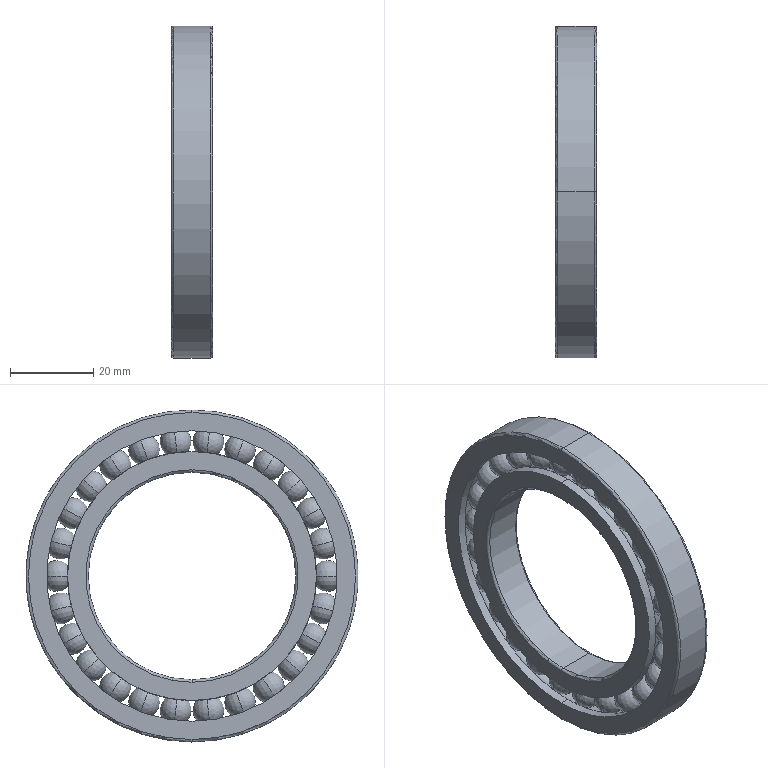Part | STEP file | deep groove ball bearings gb._Rolling bearings 16010 GB 276-94 | 1 solid | 157 faces | box 10 x 80 x 80 mm | volume 24148 mm3 | torus 89 | sphere 52 | cylinder 12 | plane 4 | commonest cylinder face diameters 60 x4 70 x4 50 x2 80 x2